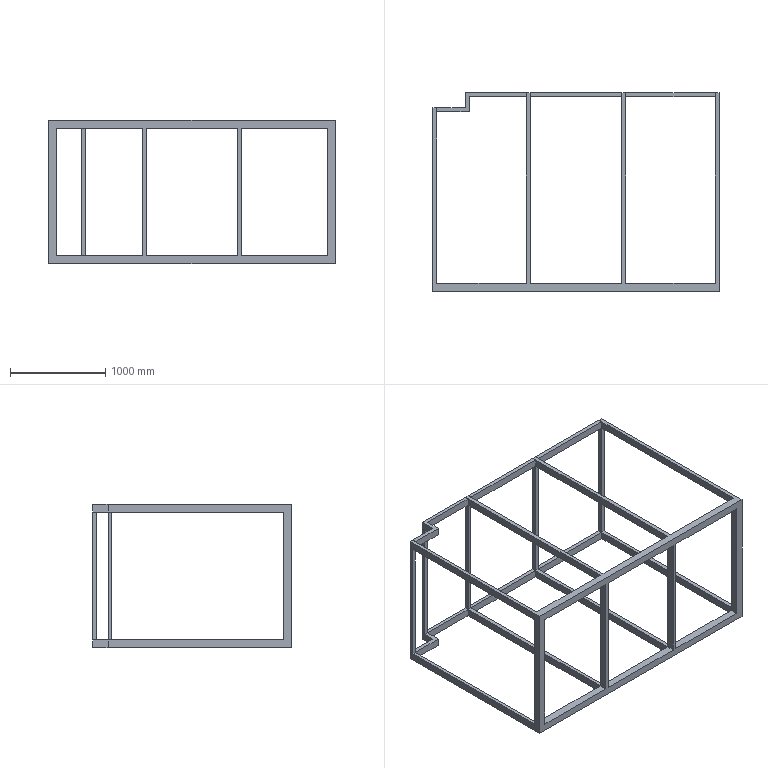Part | STEP file | 果蔬烘干机框架-111 | 12 solids | 125 faces | box 3000 x 2080 x 1500 mm | volume 144224000 mm3 | plane 125